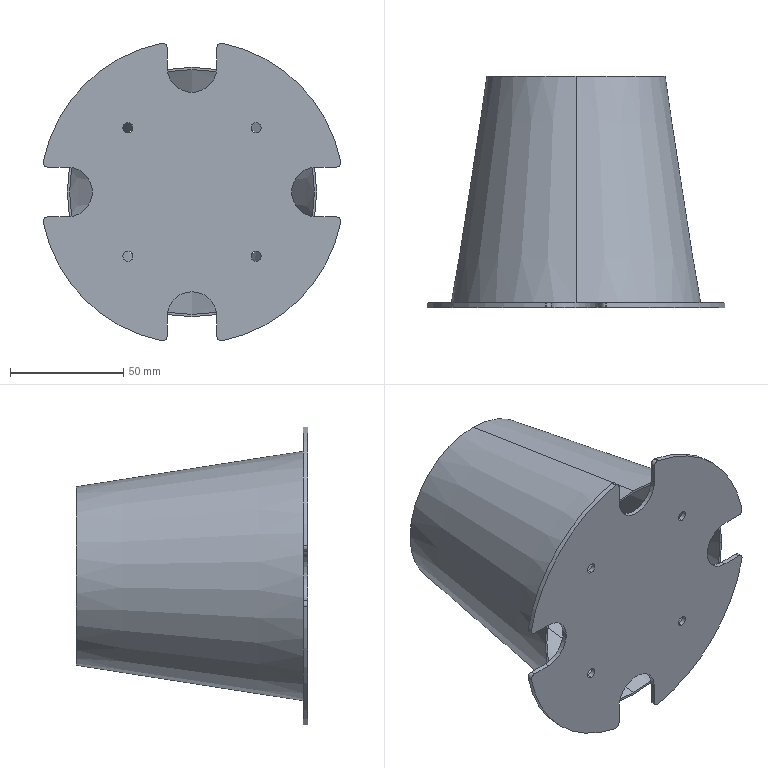Part | SolidWorks | features BaseBody 2 | 2 solids | 43 faces | box 131.373 x 102 x 131.373 mm | volume 54164 mm3 | cylinder 27 | plane 12 | cone 4 | commonest cylinder face diameters 4 x10 4.5 x8 22 x5 134 x4
STEP:
#1=CARTESIAN_POINT('',(0.,100.,38.363));
#2=VERTEX_POINT('',#1);
#3=CARTESIAN_POINT('',(0.,0.,53.988));
#4=VERTEX_POINT('',#3);
#5=CARTESIAN_POINT('',(0.,99.846,38.387));
#6=DIRECTION('',(0.,-0.988,0.1544));
#7=VECTOR('',#6,1000.);
#8=LINE('',#5,#7);
#9=EDGE_CURVE('',#2,#4,#8,.T.);
#10=ORIENTED_EDGE('',*,*,#9,.F.);
#11=CARTESIAN_POINT('',(0.,100.,-38.363));
#12=VERTEX_POINT('',#11);
#13=CARTESIAN_POINT('',(0.,100.,0.));
#14=DIRECTION('',(0.,1.,0.));
#15=DIRECTION('',(0.,0.,1.));
#16=AXIS2_PLACEMENT_3D('',#13,#14,#15);
#17=CIRCLE('',#16,38.363);
#18=EDGE_CURVE('',#2,#12,#17,.T.);
#19=ORIENTED_EDGE('',*,*,#18,.T.);
#20=CARTESIAN_POINT('',(0.,0.,-53.988));
#21=VERTEX_POINT('',#20);
#22=CARTESIAN_POINT('',(0.,99.846,-38.387));
#23=DIRECTION('',(0.,-0.988,-0.1544));
#24=VECTOR('',#23,1000.);
#25=LINE('',#22,#24);
#26=EDGE_CURVE('',#12,#21,#25,.T.);
#27=ORIENTED_EDGE('',*,*,#26,.T.);
#28=CARTESIAN_POINT('',(0.,0.,0.));
#29=DIRECTION('',(0.,1.,0.));
#30=DIRECTION('',(0.,0.,-1.));
#31=AXIS2_PLACEMENT_3D('',#28,#29,#30);
#32=CIRCLE('',#31,53.988);
#33=EDGE_CURVE('',#4,#21,#32,.T.);
#34=ORIENTED_EDGE('',*,*,#33,.F.);
#35=EDGE_LOOP('',(#10,#19,#27,#34));
#36=FACE_OUTER_BOUND('',#35,.T.);
#37=CARTESIAN_POINT('',(0.,99.846,0.));
#38=DIRECTION('',(0.,-1.,0.));
#39=DIRECTION('',(0.,0.,-1.));
#40=AXIS2_PLACEMENT_3D('',#37,#38,#39);
#41=CONICAL_SURFACE('',#40,38.387,0.155);
#42=ADVANCED_FACE('',(#36),#41,.F.);
#43=CARTESIAN_POINT('',(0.,100.,39.375));
#44=VERTEX_POINT('',#43);
#45=CARTESIAN_POINT('',(0.,0.,55.));
#46=VERTEX_POINT('',#45);
#47=CARTESIAN_POINT('',(0.,100.,39.375));
#48=DIRECTION('',(0.,-0.988,0.1544));
#49=VECTOR('',#48,1000.);
#50=LINE('',#47,#49);
#51=EDGE_CURVE('',#44,#46,#50,.T.);
#52=ORIENTED_EDGE('',*,*,#51,.F.);
#53=CARTESIAN_POINT('',(0.,100.,-39.375));
#54=VERTEX_POINT('',#53);
#55=CARTESIAN_POINT('',(0.,100.,0.));
#56=DIRECTION('',(0.,1.,0.));
#57=DIRECTION('',(0.,0.,1.));
#58=AXIS2_PLACEMENT_3D('',#55,#56,#57);
#59=CIRCLE('',#58,39.375);
#60=EDGE_CURVE('',#54,#44,#59,.T.);
#61=ORIENTED_EDGE('',*,*,#60,.F.);
#62=CARTESIAN_POINT('',(0.,0.,-55.));
#63=VERTEX_POINT('',#62);
#64=CARTESIAN_POINT('',(0.,100.,-39.375));
#65=DIRECTION('',(0.,-0.988,-0.1544));
#66=VECTOR('',#65,1000.);
#67=LINE('',#64,#66);
#68=EDGE_CURVE('',#54,#63,#67,.T.);
#69=ORIENTED_EDGE('',*,*,#68,.T.);
#70=CARTESIAN_POINT('',(0.,0.,0.));
#71=DIRECTION('',(0.,1.,0.));
#72=DIRECTION('',(0.,0.,1.));
#73=AXIS2_PLACEMENT_3D('',#70,#71,#72);
#74=CIRCLE('',#73,55.);
#75=EDGE_CURVE('',#63,#46,#74,.T.);
#76=ORIENTED_EDGE('',*,*,#75,.T.);
#77=EDGE_LOOP('',(#52,#61,#69,#76));
#78=FACE_OUTER_BOUND('',#77,.T.);
#79=CARTESIAN_POINT('',(0.,100.,0.));
#80=DIRECTION('',(0.,-1.,0.));
#81=DIRECTION('',(0.,0.,-1.));
#82=AXIS2_PLACEMENT_3D('',#79,#80,#81);
#83=CONICAL_SURFACE('',#82,39.375,0.155);
#84=ADVANCED_FACE('',(#78),#83,.T.);
#85=CARTESIAN_POINT('',(0.,100.,0.));
#86=DIRECTION('',(0.,1.,0.));
#87=DIRECTION('',(0.,0.,1.));
#88=AXIS2_PLACEMENT_3D('',#85,#86,#87);
#89=CIRCLE('',#88,38.363);
#90=EDGE_CURVE('',#12,#2,#89,.T.);
#91=ORIENTED_EDGE('',*,*,#90,.F.);
#92=ORIENTED_EDGE('',*,*,#18,.F.);
#93=EDGE_LOOP('',(#91,#92));
#94=FACE_BOUND('',#93,.T.);
#95=ORIENTED_EDGE('',*,*,#60,.T.);
#96=CARTESIAN_POINT('',(0.,100.,0.));
#97=DIRECTION('',(0.,1.,0.));
#98=DIRECTION('',(0.,0.,1.));
#99=AXIS2_PLACEMENT_3D('',#96,#97,#98);
#100=CIRCLE('',#99,39.375);
#101=EDGE_CURVE('',#44,#54,#100,.T.);
#102=ORIENTED_EDGE('',*,*,#101,.T.);
#103=EDGE_LOOP('',(#95,#102));
#104=FACE_OUTER_BOUND('',#103,.T.);
#105=CARTESIAN_POINT('',(-39.375,100.,0.));
#106=DIRECTION('',(0.,1.,0.));
#107=DIRECTION('',(1.,0.,0.));
#108=AXIS2_PLACEMENT_3D('',#105,#106,#107);
#109=PLANE('',#108);
#110=ADVANCED_FACE('',(#94,#104),#109,.T.);
#111=CARTESIAN_POINT('',(0.,0.,0.));
#112=DIRECTION('',(0.,1.,0.));
#113=DIRECTION('',(0.,0.,-1.));
#114=AXIS2_PLACEMENT_3D('',#111,#112,#113);
#115=CIRCLE('',#114,53.988);
#116=EDGE_CURVE('',#21,#4,#115,.T.);
#117=ORIENTED_EDGE('',*,*,#116,.T.);
#118=ORIENTED_EDGE('',*,*,#33,.T.);
#119=EDGE_LOOP('',(#117,#118));
#120=FACE_BOUND('',#119,.T.);
#121=ORIENTED_EDGE('',*,*,#75,.F.);
#122=CARTESIAN_POINT('',(0.,0.,0.));
#123=DIRECTION('',(0.,1.,0.));
#124=DIRECTION('',(0.,0.,1.));
#125=AXIS2_PLACEMENT_3D('',#122,#123,#124);
#126=CIRCLE('',#125,55.);
#127=EDGE_CURVE('',#46,#63,#126,.T.);
#128=ORIENTED_EDGE('',*,*,#127,.F.);
#129=EDGE_LOOP('',(#121,#128));
#130=FACE_OUTER_BOUND('',#129,.T.);
#131=CARTESIAN_POINT('',(0.,0.,0.));
#132=DIRECTION('',(0.,-1.,0.));
#133=DIRECTION('',(0.,0.,-1.));
#134=AXIS2_PLACEMENT_3D('',#131,#132,#133);
#135=PLANE('',#134);
#136=ADVANCED_FACE('',(#120,#130),#135,.T.);
#137=ORIENTED_EDGE('',*,*,#101,.F.);
#138=ORIENTED_EDGE('',*,*,#51,.T.);
#139=ORIENTED_EDGE('',*,*,#127,.T.);
#140=ORIENTED_EDGE('',*,*,#68,.F.);
#141=EDGE_LOOP('',(#137,#138,#139,#140));
#142=FACE_OUTER_BOUND('',#141,.T.);
#143=CARTESIAN_POINT('',(0.,100.,0.));
#144=DIRECTION('',(0.,-1.,0.));
#145=DIRECTION('',(0.,0.,-1.));
#146=AXIS2_PLACEMENT_3D('',#143,#144,#145);
#147=CONICAL_SURFACE('',#146,39.375,0.155);
#148=ADVANCED_FACE('',(#142),#147,.T.);
#149=ORIENTED_EDGE('',*,*,#90,.T.);
#150=ORIENTED_EDGE('',*,*,#9,.T.);
#151=ORIENTED_EDGE('',*,*,#116,.F.);
#152=ORIENTED_EDGE('',*,*,#26,.F.);
#153=EDGE_LOOP('',(#149,#150,#151,#152));
#154=FACE_OUTER_BOUND('',#153,.T.);
#155=CARTESIAN_POINT('',(0.,99.846,0.));
#156=DIRECTION('',(0.,-1.,0.));
#157=DIRECTION('',(0.,0.,-1.));
#158=AXIS2_PLACEMENT_3D('',#155,#156,#157);
#159=CONICAL_SURFACE('',#158,38.387,0.155);
#160=ADVANCED_FACE('',(#154),#159,.F.);
#161=CLOSED_SHELL('',(#42,#84,#110,#136,#148,#160));
#162=MANIFOLD_SOLID_BREP('',#161);
#163=CARTESIAN_POINT('',(13.4,0.,-65.646));
#164=VERTEX_POINT('',#163);
#165=CARTESIAN_POINT('',(11.,0.,-63.687));
#166=VERTEX_POINT('',#165);
#167=CARTESIAN_POINT('',(13.,0.,-63.687));
#168=DIRECTION('',(0.,1.,0.));
#169=DIRECTION('',(0.,0.,-1.));
#170=AXIS2_PLACEMENT_3D('',#167,#168,#169);
#171=CIRCLE('',#170,2.);
#172=EDGE_CURVE('',#164,#166,#171,.T.);
#173=ORIENTED_EDGE('',*,*,#172,.F.);
#174=CARTESIAN_POINT('',(13.4,-2.,-65.646));
#175=VERTEX_POINT('',#174);
#176=CARTESIAN_POINT('',(13.4,-2.,-65.646));
#177=DIRECTION('',(0.,1.,0.));
#178=VECTOR('',#177,1000.);
#179=LINE('',#176,#178);
#180=EDGE_CURVE('',#175,#164,#179,.T.);
#181=ORIENTED_EDGE('',*,*,#180,.F.);
#182=CARTESIAN_POINT('',(11.,-2.,-63.687));
#183=VERTEX_POINT('',#182);
#184=CARTESIAN_POINT('',(13.,-2.,-63.687));
#185=DIRECTION('',(0.,-1.,0.));
#186=DIRECTION('',(0.,0.,-1.));
#187=AXIS2_PLACEMENT_3D('',#184,#185,#186);
#188=CIRCLE('',#187,2.);
#189=EDGE_CURVE('',#183,#175,#188,.T.);
#190=ORIENTED_EDGE('',*,*,#189,.F.);
#191=CARTESIAN_POINT('',(11.,-2.001,-63.687));
#192=DIRECTION('',(0.,-1.,0.));
#193=VECTOR('',#192,1000.);
#194=LINE('',#191,#193);
#195=EDGE_CURVE('',#166,#183,#194,.T.);
#196=ORIENTED_EDGE('',*,*,#195,.F.);
#197=EDGE_LOOP('',(#173,#181,#190,#196));
#198=FACE_OUTER_BOUND('',#197,.T.);
#199=CARTESIAN_POINT('',(13.,-2.,-63.687));
#200=DIRECTION('',(0.,1.,0.));
#201=DIRECTION('',(0.,0.,1.));
#202=AXIS2_PLACEMENT_3D('',#199,#200,#201);
#203=CYLINDRICAL_SURFACE('',#202,2.);
#204=ADVANCED_FACE('',(#198),#203,.T.);
#205=CARTESIAN_POINT('',(-13.4,-2.,-65.646));
#206=VERTEX_POINT('',#205);
#207=CARTESIAN_POINT('',(-11.,-2.,-63.687));
#208=VERTEX_POINT('',#207);
#209=CARTESIAN_POINT('',(-13.,-2.,-63.687));
#210=DIRECTION('',(0.,-1.,0.));
#211=DIRECTION('',(0.,0.,-1.));
#212=AXIS2_PLACEMENT_3D('',#209,#210,#211);
#213=CIRCLE('',#212,2.);
#214=EDGE_CURVE('',#206,#208,#213,.T.);
#215=ORIENTED_EDGE('',*,*,#214,.F.);
#216=CARTESIAN_POINT('',(-13.4,0.,-65.646));
#217=VERTEX_POINT('',#216);
#218=CARTESIAN_POINT('',(-13.4,-2.,-65.646));
#219=DIRECTION('',(0.,-1.,0.));
#220=VECTOR('',#219,1000.);
#221=LINE('',#218,#220);
#222=EDGE_CURVE('',#217,#206,#221,.T.);
#223=ORIENTED_EDGE('',*,*,#222,.F.);
#224=CARTESIAN_POINT('',(-11.,0.,-63.687));
#225=VERTEX_POINT('',#224);
#226=CARTESIAN_POINT('',(-13.,0.,-63.687));
#227=DIRECTION('',(0.,1.,0.));
#228=DIRECTION('',(0.,0.,-1.));
#229=AXIS2_PLACEMENT_3D('',#226,#227,#228);
#230=CIRCLE('',#229,2.);
#231=EDGE_CURVE('',#225,#217,#230,.T.);
#232=ORIENTED_EDGE('',*,*,#231,.F.);
#233=CARTESIAN_POINT('',(-11.,-2.001,-63.687));
#234=DIRECTION('',(0.,1.,0.));
#235=VECTOR('',#234,1000.);
#236=LINE('',#233,#235);
#237=EDGE_CURVE('',#208,#225,#236,.T.);
#238=ORIENTED_EDGE('',*,*,#237,.F.);
#239=EDGE_LOOP('',(#215,#223,#232,#238));
#240=FACE_OUTER_BOUND('',#239,.T.);
#241=CARTESIAN_POINT('',(-13.,-2.,-63.687));
#242=DIRECTION('',(0.,1.,0.));
#243=DIRECTION('',(0.,0.,1.));
#244=AXIS2_PLACEMENT_3D('',#241,#242,#243);
#245=CYLINDRICAL_SURFACE('',#244,2.);
#246=ADVANCED_FACE('',(#240),#245,.T.);
#247=CARTESIAN_POINT('',(65.646,-2.,-13.4));
#248=VERTEX_POINT('',#247);
#249=CARTESIAN_POINT('',(63.687,-2.,-11.));
#250=VERTEX_POINT('',#249);
#251=CARTESIAN_POINT('',(63.687,-2.,-13.));
#252=DIRECTION('',(0.,-1.,0.));
#253=DIRECTION('',(0.,0.,-1.));
#254=AXIS2_PLACEMENT_3D('',#251,#252,#253);
#255=CIRCLE('',#254,2.);
#256=EDGE_CURVE('',#248,#250,#255,.T.);
#257=ORIENTED_EDGE('',*,*,#256,.F.);
#258=CARTESIAN_POINT('',(65.646,0.,-13.4));
#259=VERTEX_POINT('',#258);
#260=CARTESIAN_POINT('',(65.646,-2.,-13.4));
#261=DIRECTION('',(0.,-1.,0.));
#262=VECTOR('',#261,1000.);
#263=LINE('',#260,#262);
#264=EDGE_CURVE('',#259,#248,#263,.T.);
#265=ORIENTED_EDGE('',*,*,#264,.F.);
#266=CARTESIAN_POINT('',(63.687,0.,-11.));
#267=VERTEX_POINT('',#266);
#268=CARTESIAN_POINT('',(63.687,0.,-13.));
#269=DIRECTION('',(0.,1.,0.));
#270=DIRECTION('',(0.,0.,-1.));
#271=AXIS2_PLACEMENT_3D('',#268,#269,#270);
#272=CIRCLE('',#271,2.);
#273=EDGE_CURVE('',#267,#259,#272,.T.);
#274=ORIENTED_EDGE('',*,*,#273,.F.);
#275=CARTESIAN_POINT('',(63.687,-2.001,-11.));
#276=DIRECTION('',(0.,1.,0.));
#277=VECTOR('',#276,1000.);
#278=LINE('',#275,#277);
#279=EDGE_CURVE('',#250,#267,#278,.T.);
#280=ORIENTED_EDGE('',*,*,#279,.F.);
#281=EDGE_LOOP('',(#257,#265,#274,#280));
#282=FACE_OUTER_BOUND('',#281,.T.);
#283=CARTESIAN_POINT('',(63.687,-2.,-13.));
#284=DIRECTION('',(0.,1.,0.));
#285=DIRECTION('',(0.,0.,1.));
#286=AXIS2_PLACEMENT_3D('',#283,#284,#285);
#287=CYLINDRICAL_SURFACE('',#286,2.);
#288=ADVANCED_FACE('',(#282),#287,.T.);
#289=CARTESIAN_POINT('',(65.646,0.,13.4));
#290=VERTEX_POINT('',#289);
#291=CARTESIAN_POINT('',(63.687,0.,11.));
#292=VERTEX_POINT('',#291);
#293=CARTESIAN_POINT('',(63.687,0.,13.));
#294=DIRECTION('',(0.,1.,0.));
#295=DIRECTION('',(0.,0.,-1.));
#296=AXIS2_PLACEMENT_3D('',#293,#294,#295);
#297=CIRCLE('',#296,2.);
#298=EDGE_CURVE('',#290,#292,#297,.T.);
#299=ORIENTED_EDGE('',*,*,#298,.F.);
#300=CARTESIAN_POINT('',(65.646,-2.,13.4));
#301=VERTEX_POINT('',#300);
#302=CARTESIAN_POINT('',(65.646,-2.,13.4));
#303=DIRECTION('',(0.,1.,0.));
#304=VECTOR('',#303,1000.);
#305=LINE('',#302,#304);
#306=EDGE_CURVE('',#301,#290,#305,.T.);
#307=ORIENTED_EDGE('',*,*,#306,.F.);
#308=CARTESIAN_POINT('',(63.687,-2.,11.));
#309=VERTEX_POINT('',#308);
#310=CARTESIAN_POINT('',(63.687,-2.,13.));
#311=DIRECTION('',(0.,-1.,0.));
#312=DIRECTION('',(0.,0.,-1.));
#313=AXIS2_PLACEMENT_3D('',#310,#311,#312);
#314=CIRCLE('',#313,2.);
#315=EDGE_CURVE('',#309,#301,#314,.T.);
#316=ORIENTED_EDGE('',*,*,#315,.F.);
#317=CARTESIAN_POINT('',(63.687,-2.001,11.));
#318=DIRECTION('',(0.,-1.,0.));
#319=VECTOR('',#318,1000.);
#320=LINE('',#317,#319);
#321=EDGE_CURVE('',#292,#309,#320,.T.);
#322=ORIENTED_EDGE('',*,*,#321,.F.);
#323=EDGE_LOOP('',(#299,#307,#316,#322));
#324=FACE_OUTER_BOUND('',#323,.T.);
#325=CARTESIAN_POINT('',(63.687,-2.,13.));
#326=DIRECTION('',(0.,1.,0.));
#327=DIRECTION('',(0.,0.,1.));
#328=AXIS2_PLACEMENT_3D('',#325,#326,#327);
#329=CYLINDRICAL_SURFACE('',#328,2.);
#330=ADVANCED_FACE('',(#324),#329,.T.);
#331=CARTESIAN_POINT('',(-65.646,0.,-13.4));
#332=VERTEX_POINT('',#331);
#333=CARTESIAN_POINT('',(-63.687,0.,-11.));
#334=VERTEX_POINT('',#333);
#335=CARTESIAN_POINT('',(-63.687,0.,-13.));
#336=DIRECTION('',(0.,1.,0.));
#337=DIRECTION('',(0.,0.,-1.));
#338=AXIS2_PLACEMENT_3D('',#335,#336,#337);
#339=CIRCLE('',#338,2.);
#340=EDGE_CURVE('',#332,#334,#339,.T.);
#341=ORIENTED_EDGE('',*,*,#340,.F.);
#342=CARTESIAN_POINT('',(-65.646,-2.,-13.4));
#343=VERTEX_POINT('',#342);
#344=CARTESIAN_POINT('',(-65.646,-2.,-13.4));
#345=DIRECTION('',(0.,1.,0.));
#346=VECTOR('',#345,1000.);
#347=LINE('',#344,#346);
#348=EDGE_CURVE('',#343,#332,#347,.T.);
#349=ORIENTED_EDGE('',*,*,#348,.F.);
#350=CARTESIAN_POINT('',(-63.687,-2.,-11.));
#351=VERTEX_POINT('',#350);
#352=CARTESIAN_POINT('',(-63.687,-2.,-13.));
#353=DIRECTION('',(0.,-1.,0.));
#354=DIRECTION('',(0.,0.,-1.));
#355=AXIS2_PLACEMENT_3D('',#352,#353,#354);
#356=CIRCLE('',#355,2.);
#357=EDGE_CURVE('',#351,#343,#356,.T.);
#358=ORIENTED_EDGE('',*,*,#357,.F.);
#359=CARTESIAN_POINT('',(-63.687,-2.001,-11.));
#360=DIRECTION('',(0.,-1.,0.));
#361=VECTOR('',#360,1000.);
#362=LINE('',#359,#361);
#363=EDGE_CURVE('',#334,#351,#362,.T.);
#364=ORIENTED_EDGE('',*,*,#363,.F.);
#365=EDGE_LOOP('',(#341,#349,#358,#364));
#366=FACE_OUTER_BOUND('',#365,.T.);
#367=CARTESIAN_POINT('',(-63.687,-2.,-13.));
#368=DIRECTION('',(0.,1.,0.));
#369=DIRECTION('',(0.,0.,1.));
#370=AXIS2_PLACEMENT_3D('',#367,#368,#369);
#371=CYLINDRICAL_SURFACE('',#370,2.);
#372=ADVANCED_FACE('',(#366),#371,.T.);
#373=CARTESIAN_POINT('',(-65.646,-2.,13.4));
#374=VERTEX_POINT('',#373);
#375=CARTESIAN_POINT('',(-63.687,-2.,11.));
#376=VERTEX_POINT('',#375);
#377=CARTESIAN_POINT('',(-63.687,-2.,13.));
#378=DIRECTION('',(0.,-1.,0.));
#379=DIRECTION('',(0.,0.,-1.));
#380=AXIS2_PLACEMENT_3D('',#377,#378,#379);
#381=CIRCLE('',#380,2.);
#382=EDGE_CURVE('',#374,#376,#381,.T.);
#383=ORIENTED_EDGE('',*,*,#382,.F.);
#384=CARTESIAN_POINT('',(-65.646,0.,13.4));
#385=VERTEX_POINT('',#384);
#386=CARTESIAN_POINT('',(-65.646,-2.,13.4));
#387=DIRECTION('',(0.,-1.,0.));
#388=VECTOR('',#387,1000.);
#389=LINE('',#386,#388);
#390=EDGE_CURVE('',#385,#374,#389,.T.);
#391=ORIENTED_EDGE('',*,*,#390,.F.);
#392=CARTESIAN_POINT('',(-63.687,0.,11.));
#393=VERTEX_POINT('',#392);
#394=CARTESIAN_POINT('',(-63.687,0.,13.));
#395=DIRECTION('',(0.,1.,0.));
#396=DIRECTION('',(0.,0.,-1.));
#397=AXIS2_PLACEMENT_3D('',#394,#395,#396);
#398=CIRCLE('',#397,2.);
#399=EDGE_CURVE('',#393,#385,#398,.T.);
#400=ORIENTED_EDGE('',*,*,#399,.F.);
#401=CARTESIAN_POINT('',(-63.687,-2.001,11.));
#402=DIRECTION('',(0.,1.,0.));
#403=VECTOR('',#402,1000.);
#404=LINE('',#401,#403);
#405=EDGE_CURVE('',#376,#393,#404,.T.);
#406=ORIENTED_EDGE('',*,*,#405,.F.);
#407=EDGE_LOOP('',(#383,#391,#400,#406));
#408=FACE_OUTER_BOUND('',#407,.T.);
#409=CARTESIAN_POINT('',(-63.687,-2.,13.));
#410=DIRECTION('',(0.,1.,0.));
#411=DIRECTION('',(0.,0.,1.));
#412=AXIS2_PLACEMENT_3D('',#409,#410,#411);
#413=CYLINDRICAL_SURFACE('',#412,2.);
#414=ADVANCED_FACE('',(#408),#413,.T.);
#415=CARTESIAN_POINT('',(13.,-2.,65.687));
#416=VERTEX_POINT('',#415);
#417=CARTESIAN_POINT('',(13.,0.,65.687));
#418=VERTEX_POINT('',#417);
#419=CARTESIAN_POINT('',(13.,-2.,65.687));
#420=DIRECTION('',(0.,1.,0.));
#421=VECTOR('',#420,1000.);
#422=LINE('',#419,#421);
#423=EDGE_CURVE('',#416,#418,#422,.T.);
#424=ORIENTED_EDGE('',*,*,#423,.F.);
#425=CARTESIAN_POINT('',(13.4,-2.,65.646));
#426=VERTEX_POINT('',#425);
#427=CARTESIAN_POINT('',(13.,-2.,63.687));
#428=DIRECTION('',(0.,-1.,0.));
#429=DIRECTION('',(0.,0.,-1.));
#430=AXIS2_PLACEMENT_3D('',#427,#428,#429);
#431=CIRCLE('',#430,2.);
#432=EDGE_CURVE('',#426,#416,#431,.T.);
#433=ORIENTED_EDGE('',*,*,#432,.F.);
#434=CARTESIAN_POINT('',(13.4,0.,65.646));
#435=VERTEX_POINT('',#434);
#436=CARTESIAN_POINT('',(13.4,-2.,65.646));
#437=DIRECTION('',(0.,-1.,0.));
#438=VECTOR('',#437,1000.);
#439=LINE('',#436,#438);
#440=EDGE_CURVE('',#435,#426,#439,.T.);
#441=ORIENTED_EDGE('',*,*,#440,.F.);
#442=CARTESIAN_POINT('',(13.,0.,63.687));
#443=DIRECTION('',(0.,1.,0.));
#444=DIRECTION('',(0.,0.,-1.));
#445=AXIS2_PLACEMENT_3D('',#442,#443,#444);
#446=CIRCLE('',#445,2.);
#447=EDGE_CURVE('',#418,#435,#446,.T.);
#448=ORIENTED_EDGE('',*,*,#447,.F.);
#449=EDGE_LOOP('',(#424,#433,#441,#448));
#450=FACE_OUTER_BOUND('',#449,.T.);
#451=CARTESIAN_POINT('',(13.,-2.,63.687));
#452=DIRECTION('',(0.,1.,0.));
#453=DIRECTION('',(0.,0.,1.));
#454=AXIS2_PLACEMENT_3D('',#451,#452,#453);
#455=CYLINDRICAL_SURFACE('',#454,2.);
#456=ADVANCED_FACE('',(#450),#455,.T.);
#457=CARTESIAN_POINT('',(-13.,-2.,65.687));
#458=VERTEX_POINT('',#457);
#459=CARTESIAN_POINT('',(-13.,0.,65.687));
#460=VERTEX_POINT('',#459);
#461=CARTESIAN_POINT('',(-13.,-2.,65.687));
#462=DIRECTION('',(0.,1.,0.));
#463=VECTOR('',#462,1000.);
#464=LINE('',#461,#463);
#465=EDGE_CURVE('',#458,#460,#464,.T.);
#466=ORIENTED_EDGE('',*,*,#465,.F.);
#467=CARTESIAN_POINT('',(-11.,-2.,63.687));
#468=VERTEX_POINT('',#467);
#469=CARTESIAN_POINT('',(-13.,-2.,63.687));
#470=DIRECTION('',(0.,-1.,0.));
#471=DIRECTION('',(0.,0.,-1.));
#472=AXIS2_PLACEMENT_3D('',#469,#470,#471);
#473=CIRCLE('',#472,2.);
#474=EDGE_CURVE('',#468,#458,#473,.T.);
#475=ORIENTED_EDGE('',*,*,#474,.F.);
#476=CARTESIAN_POINT('',(-11.,0.,63.687));
#477=VERTEX_POINT('',#476);
#478=CARTESIAN_POINT('',(-11.,-2.001,63.687));
#479=DIRECTION('',(0.,-1.,0.));
#480=VECTOR('',#479,1000.);
#481=LINE('',#478,#480);
#482=EDGE_CURVE('',#477,#468,#481,.T.);
#483=ORIENTED_EDGE('',*,*,#482,.F.);
#484=CARTESIAN_POINT('',(-13.,0.,63.687));
#485=DIRECTION('',(0.,1.,0.));
#486=DIRECTION('',(0.,0.,-1.));
#487=AXIS2_PLACEMENT_3D('',#484,#485,#486);
#488=CIRCLE('',#487,2.);
#489=EDGE_CURVE('',#460,#477,#488,.T.);
#490=ORIENTED_EDGE('',*,*,#489,.F.);
#491=EDGE_LOOP('',(#466,#475,#483,#490));
#492=FACE_OUTER_BOUND('',#491,.T.);
#493=CARTESIAN_POINT('',(-13.,-2.,63.687));
#494=DIRECTION('',(0.,1.,0.));
#495=DIRECTION('',(0.,0.,1.));
#496=AXIS2_PLACEMENT_3D('',#493,#494,#495);
#497=CYLINDRICAL_SURFACE('',#496,2.);
#498=ADVANCED_FACE('',(#492),#497,.T.);
#499=CARTESIAN_POINT('',(55.,-2.,-11.));
#500=VERTEX_POINT('',#499);
#501=CARTESIAN_POINT('',(55.,0.,-11.));
#502=VERTEX_POINT('',#501);
#503=CARTESIAN_POINT('',(55.,-2.001,-11.));
#504=DIRECTION('',(0.,1.,0.));
#505=VECTOR('',#504,1000.);
#506=LINE('',#503,#505);
#507=EDGE_CURVE('',#500,#502,#506,.T.);
#508=ORIENTED_EDGE('',*,*,#507,.T.);
#509=CARTESIAN_POINT('',(55.,0.,11.));
#510=VERTEX_POINT('',#509);
#511=CARTESIAN_POINT('',(55.,0.,0.));
#512=DIRECTION('',(0.,1.,0.));
#513=DIRECTION('',(-1.,0.,0.));
#514=AXIS2_PLACEMENT_3D('',#511,#512,#513);
#515=CIRCLE('',#514,11.);
#516=EDGE_CURVE('',#502,#510,#515,.T.);
#517=ORIENTED_EDGE('',*,*,#516,.T.);
#518=CARTESIAN_POINT('',(55.,-2.,11.));
#519=VERTEX_POINT('',#518);
#520=CARTESIAN_POINT('',(55.,-2.001,11.));
#521=DIRECTION('',(0.,1.,0.));
#522=VECTOR('',#521,1000.);
#523=LINE('',#520,#522);
#524=EDGE_CURVE('',#519,#510,#523,.T.);
#525=ORIENTED_EDGE('',*,*,#524,.F.);
#526=CARTESIAN_POINT('',(55.,-2.,0.));
#527=DIRECTION('',(0.,1.,0.));
#528=DIRECTION('',(0.,0.,-1.));
#529=AXIS2_PLACEMENT_3D('',#526,#527,#528);
#530=CIRCLE('',#529,11.);
#531=EDGE_CURVE('',#500,#519,#530,.T.);
#532=ORIENTED_EDGE('',*,*,#531,.F.);
#533=EDGE_LOOP('',(#508,#517,#525,#532));
#534=FACE_OUTER_BOUND('',#533,.T.);
#535=CARTESIAN_POINT('',(55.,-2.001,0.));
#536=DIRECTION('',(0.,1.,0.));
#537=DIRECTION('',(0.,0.,1.));
#538=AXIS2_PLACEMENT_3D('',#535,#536,#537);
#539=CYLINDRICAL_SURFACE('',#538,11.);
#540=ADVANCED_FACE('',(#534),#539,.F.);
#541=CARTESIAN_POINT('',(67.,-2.,-11.));
#542=DIRECTION('',(-1.,0.,0.));
#543=VECTOR('',#542,1000.);
#544=LINE('',#541,#543);
#545=EDGE_CURVE('',#250,#500,#544,.T.);
#546=ORIENTED_EDGE('',*,*,#545,.F.);
#547=ORIENTED_EDGE('',*,*,#279,.T.);
#548=CARTESIAN_POINT('',(67.,0.,-11.));
#549=DIRECTION('',(-1.,0.,0.));
#550=VECTOR('',#549,1000.);
#551=LINE('',#548,#550);
#552=EDGE_CURVE('',#267,#502,#551,.T.);
#553=ORIENTED_EDGE('',*,*,#552,.T.);
#554=ORIENTED_EDGE('',*,*,#507,.F.);
#555=EDGE_LOOP('',(#546,#547,#553,#554));
#556=FACE_OUTER_BOUND('',#555,.T.);
#557=CARTESIAN_POINT('',(67.,-2.001,-11.));
#558=DIRECTION('',(0.,0.,-1.));
#559=DIRECTION('',(0.,-1.,0.));
#560=AXIS2_PLACEMENT_3D('',#557,#558,#559);
#561=PLANE('',#560);
#562=ADVANCED_FACE('',(#556),#561,.F.);
#563=CARTESIAN_POINT('',(67.,0.,11.));
#564=DIRECTION('',(1.,0.,0.));
#565=VECTOR('',#564,1000.);
#566=LINE('',#563,#565);
#567=EDGE_CURVE('',#510,#292,#566,.T.);
#568=ORIENTED_EDGE('',*,*,#567,.T.);
#569=ORIENTED_EDGE('',*,*,#321,.T.);
#570=CARTESIAN_POINT('',(67.,-2.,11.));
#571=DIRECTION('',(1.,0.,0.));
#572=VECTOR('',#571,1000.);
#573=LINE('',#570,#572);
#574=EDGE_CURVE('',#519,#309,#573,.T.);
#575=ORIENTED_EDGE('',*,*,#574,.F.);
#576=ORIENTED_EDGE('',*,*,#524,.T.);
#577=EDGE_LOOP('',(#568,#569,#575,#576));
#578=FACE_OUTER_BOUND('',#577,.T.);
#579=CARTESIAN_POINT('',(67.,-2.001,11.));
#580=DIRECTION('',(0.,0.,1.));
#581=DIRECTION('',(1.,0.,0.));
#582=AXIS2_PLACEMENT_3D('',#579,#580,#581);
#583=PLANE('',#582);
#584=ADVANCED_FACE('',(#578),#583,.F.);
#585=CARTESIAN_POINT('',(11.,-2.,55.));
#586=VERTEX_POINT('',#585);
#587=CARTESIAN_POINT('',(11.,0.,55.));
#588=VERTEX_POINT('',#587);
#589=CARTESIAN_POINT('',(11.,-2.001,55.));
#590=DIRECTION('',(0.,1.,0.));
#591=VECTOR('',#590,1000.);
#592=LINE('',#589,#591);
#593=EDGE_CURVE('',#586,#588,#592,.T.);
#594=ORIENTED_EDGE('',*,*,#593,.T.);
#595=CARTESIAN_POINT('',(-11.,0.,55.));
#596=VERTEX_POINT('',#595);
#597=CARTESIAN_POINT('',(0.,0.,55.));
#598=DIRECTION('',(0.,1.,0.));
#599=DIRECTION('',(0.,0.,-1.));
#600=AXIS2_PLACEMENT_3D('',#597,#598,#599);
#601=CIRCLE('',#600,11.);
#602=EDGE_CURVE('',#588,#596,#601,.T.);
#603=ORIENTED_EDGE('',*,*,#602,.T.);
#604=CARTESIAN_POINT('',(-11.,-2.,55.));
#605=VERTEX_POINT('',#604);
#606=CARTESIAN_POINT('',(-11.,-2.001,55.));
#607=DIRECTION('',(0.,1.,0.));
#608=VECTOR('',#607,1000.);
#609=LINE('',#606,#608);
#610=EDGE_CURVE('',#605,#596,#609,.T.);
#611=ORIENTED_EDGE('',*,*,#610,.F.);
#612=CARTESIAN_POINT('',(0.,-2.,55.));
#613=DIRECTION('',(0.,1.,0.));
#614=DIRECTION('',(0.,0.,-1.));
#615=AXIS2_PLACEMENT_3D('',#612,#613,#614);
#616=CIRCLE('',#615,11.);
#617=EDGE_CURVE('',#586,#605,#616,.T.);
#618=ORIENTED_EDGE('',*,*,#617,.F.);
#619=EDGE_LOOP('',(#594,#603,#611,#618));
#620=FACE_OUTER_BOUND('',#619,.T.);
#621=CARTESIAN_POINT('',(0.,-2.001,55.));
#622=DIRECTION('',(0.,1.,0.));
#623=DIRECTION('',(0.,0.,1.));
#624=AXIS2_PLACEMENT_3D('',#621,#622,#623);
#625=CYLINDRICAL_SURFACE('',#624,11.);
#626=ADVANCED_FACE('',(#620),#625,.F.);
#627=CARTESIAN_POINT('',(11.,-2.,63.687));
#628=VERTEX_POINT('',#627);
#629=CARTESIAN_POINT('',(11.,-2.,67.));
#630=DIRECTION('',(0.,0.,-1.));
#631=VECTOR('',#630,1000.);
#632=LINE('',#629,#631);
#633=EDGE_CURVE('',#628,#586,#632,.T.);
#634=ORIENTED_EDGE('',*,*,#633,.F.);
#635=CARTESIAN_POINT('',(11.,0.,63.687));
#636=VERTEX_POINT('',#635);
#637=CARTESIAN_POINT('',(11.,-2.001,63.687));
#638=DIRECTION('',(0.,1.,0.));
#639=VECTOR('',#638,1000.);
#640=LINE('',#637,#639);
#641=EDGE_CURVE('',#628,#636,#640,.T.);
#642=ORIENTED_EDGE('',*,*,#641,.T.);
#643=CARTESIAN_POINT('',(11.,0.,67.));
#644=DIRECTION('',(0.,0.,-1.));
#645=VECTOR('',#644,1000.);
#646=LINE('',#643,#645);
#647=EDGE_CURVE('',#636,#588,#646,.T.);
#648=ORIENTED_EDGE('',*,*,#647,.T.);
#649=ORIENTED_EDGE('',*,*,#593,.F.);
#650=EDGE_LOOP('',(#634,#642,#648,#649));
#651=FACE_OUTER_BOUND('',#650,.T.);
#652=CARTESIAN_POINT('',(11.,-2.001,67.));
#653=DIRECTION('',(1.,0.,0.));
#654=DIRECTION('',(0.,1.,0.));
#655=AXIS2_PLACEMENT_3D('',#652,#653,#654);
#656=PLANE('',#655);
#657=ADVANCED_FACE('',(#651),#656,.F.);
#658=CARTESIAN_POINT('',(-11.,0.,67.));
#659=DIRECTION('',(0.,0.,1.));
#660=VECTOR('',#659,1000.);
#661=LINE('',#658,#660);
#662=EDGE_CURVE('',#596,#477,#661,.T.);
#663=ORIENTED_EDGE('',*,*,#662,.T.);
#664=ORIENTED_EDGE('',*,*,#482,.T.);
#665=CARTESIAN_POINT('',(-11.,-2.,67.));
#666=DIRECTION('',(0.,0.,1.));
#667=VECTOR('',#666,1000.);
#668=LINE('',#665,#667);
#669=EDGE_CURVE('',#605,#468,#668,.T.);
#670=ORIENTED_EDGE('',*,*,#669,.F.);
#671=ORIENTED_EDGE('',*,*,#610,.T.);
#672=EDGE_LOOP('',(#663,#664,#670,#671));
#673=FACE_OUTER_BOUND('',#672,.T.);
#674=CARTESIAN_POINT('',(-11.,-2.001,67.));
#675=DIRECTION('',(-1.,0.,0.));
#676=DIRECTION('',(0.,0.,1.));
#677=AXIS2_PLACEMENT_3D('',#674,#675,#676);
#678=PLANE('',#677);
#679=ADVANCED_FACE('',(#673),#678,.F.);
#680=CARTESIAN_POINT('',(-55.,-2.,11.));
#681=VERTEX_POINT('',#680);
#682=CARTESIAN_POINT('',(-55.,0.,11.));
#683=VERTEX_POINT('',#682);
#684=CARTESIAN_POINT('',(-55.,-2.001,11.));
#685=DIRECTION('',(0.,1.,0.));
#686=VECTOR('',#685,1000.);
#687=LINE('',#684,#686);
#688=EDGE_CURVE('',#681,#683,#687,.T.);
#689=ORIENTED_EDGE('',*,*,#688,.T.);
#690=CARTESIAN_POINT('',(-55.,0.,-11.));
#691=VERTEX_POINT('',#690);
#692=CARTESIAN_POINT('',(-55.,0.,0.));
#693=DIRECTION('',(0.,1.,0.));
#694=DIRECTION('',(1.,0.,0.));
#695=AXIS2_PLACEMENT_3D('',#692,#693,#694);
#696=CIRCLE('',#695,11.);
#697=EDGE_CURVE('',#683,#691,#696,.T.);
#698=ORIENTED_EDGE('',*,*,#697,.T.);
#699=CARTESIAN_POINT('',(-55.,-2.,-11.));
#700=VERTEX_POINT('',#699);
#701=CARTESIAN_POINT('',(-55.,-2.001,-11.));
#702=DIRECTION('',(0.,1.,0.));
#703=VECTOR('',#702,1000.);
#704=LINE('',#701,#703);
#705=EDGE_CURVE('',#700,#691,#704,.T.);
#706=ORIENTED_EDGE('',*,*,#705,.F.);
#707=CARTESIAN_POINT('',(-55.,-2.,0.));
#708=DIRECTION('',(0.,1.,0.));
#709=DIRECTION('',(0.,0.,-1.));
#710=AXIS2_PLACEMENT_3D('',#707,#708,#709);
#711=CIRCLE('',#710,11.);
#712=EDGE_CURVE('',#681,#700,#711,.T.);
#713=ORIENTED_EDGE('',*,*,#712,.F.);
#714=EDGE_LOOP('',(#689,#698,#706,#713));
#715=FACE_OUTER_BOUND('',#714,.T.);
#716=CARTESIAN_POINT('',(-55.,-2.001,0.));
#717=DIRECTION('',(0.,1.,0.));
#718=DIRECTION('',(0.,0.,1.));
#719=AXIS2_PLACEMENT_3D('',#716,#717,#718);
#720=CYLINDRICAL_SURFACE('',#719,11.);
#721=ADVANCED_FACE('',(#715),#720,.F.);
#722=CARTESIAN_POINT('',(-67.,-2.,11.));
#723=DIRECTION('',(1.,0.,0.));
#724=VECTOR('',#723,1000.);
#725=LINE('',#722,#724);
#726=EDGE_CURVE('',#376,#681,#725,.T.);
#727=ORIENTED_EDGE('',*,*,#726,.F.);
#728=ORIENTED_EDGE('',*,*,#405,.T.);
#729=CARTESIAN_POINT('',(-67.,0.,11.));
#730=DIRECTION('',(1.,0.,0.));
#731=VECTOR('',#730,1000.);
#732=LINE('',#729,#731);
#733=EDGE_CURVE('',#393,#683,#732,.T.);
#734=ORIENTED_EDGE('',*,*,#733,.T.);
#735=ORIENTED_EDGE('',*,*,#688,.F.);
#736=EDGE_LOOP('',(#727,#728,#734,#735));
#737=FACE_OUTER_BOUND('',#736,.T.);
#738=CARTESIAN_POINT('',(-67.,-2.001,11.));
#739=DIRECTION('',(0.,0.,1.));
#740=DIRECTION('',(1.,0.,0.));
#741=AXIS2_PLACEMENT_3D('',#738,#739,#740);
#742=PLANE('',#741);
#743=ADVANCED_FACE('',(#737),#742,.F.);
#744=CARTESIAN_POINT('',(-67.,0.,-11.));
#745=DIRECTION('',(-1.,0.,0.));
#746=VECTOR('',#745,1000.);
#747=LINE('',#744,#746);
#748=EDGE_CURVE('',#691,#334,#747,.T.);
#749=ORIENTED_EDGE('',*,*,#748,.T.);
#750=ORIENTED_EDGE('',*,*,#363,.T.);
#751=CARTESIAN_POINT('',(-67.,-2.,-11.));
#752=DIRECTION('',(-1.,0.,0.));
#753=VECTOR('',#752,1000.);
#754=LINE('',#751,#753);
#755=EDGE_CURVE('',#700,#351,#754,.T.);
#756=ORIENTED_EDGE('',*,*,#755,.F.);
#757=ORIENTED_EDGE('',*,*,#705,.T.);
#758=EDGE_LOOP('',(#749,#750,#756,#757));
#759=FACE_OUTER_BOUND('',#758,.T.);
#760=CARTESIAN_POINT('',(-67.,-2.001,-11.));
#761=DIRECTION('',(0.,0.,-1.));
#762=DIRECTION('',(0.,-1.,0.));
#763=AXIS2_PLACEMENT_3D('',#760,#761,#762);
#764=PLANE('',#763);
#765=ADVANCED_FACE('',(#759),#764,.F.);
#766=CARTESIAN_POINT('',(0.,-2.,-44.));
#767=VERTEX_POINT('',#766);
#768=CARTESIAN_POINT('',(0.,0.,-44.));
#769=VERTEX_POINT('',#768);
#770=CARTESIAN_POINT('',(0.,-2.001,-44.));
#771=DIRECTION('',(0.,1.,0.));
#772=VECTOR('',#771,1000.);
#773=LINE('',#770,#772);
#774=EDGE_CURVE('',#767,#769,#773,.T.);
#775=ORIENTED_EDGE('',*,*,#774,.F.);
#776=CARTESIAN_POINT('',(-11.,-2.,-55.));
#777=VERTEX_POINT('',#776);
#778=CARTESIAN_POINT('',(0.,-2.,-55.));
#779=DIRECTION('',(0.,1.,0.));
#780=DIRECTION('',(0.,0.,-1.));
#781=AXIS2_PLACEMENT_3D('',#778,#779,#780);
#782=CIRCLE('',#781,11.);
#783=EDGE_CURVE('',#777,#767,#782,.T.);
#784=ORIENTED_EDGE('',*,*,#783,.F.);
#785=CARTESIAN_POINT('',(-11.,0.,-55.));
#786=VERTEX_POINT('',#785);
#787=CARTESIAN_POINT('',(-11.,-2.001,-55.));
#788=DIRECTION('',(0.,1.,0.));
#789=VECTOR('',#788,1000.);
#790=LINE('',#787,#789);
#791=EDGE_CURVE('',#777,#786,#790,.T.);
#792=ORIENTED_EDGE('',*,*,#791,.T.);
#793=CARTESIAN_POINT('',(0.,0.,-55.));
#794=DIRECTION('',(0.,1.,0.));
#795=DIRECTION('',(0.,0.,1.));
#796=AXIS2_PLACEMENT_3D('',#793,#794,#795);
#797=CIRCLE('',#796,11.);
#798=EDGE_CURVE('',#786,#769,#797,.T.);
#799=ORIENTED_EDGE('',*,*,#798,.T.);
#800=EDGE_LOOP('',(#775,#784,#792,#799));
#801=FACE_OUTER_BOUND('',#800,.T.);
#802=CARTESIAN_POINT('',(0.,-2.001,-55.));
#803=DIRECTION('',(0.,1.,0.));
#804=DIRECTION('',(0.,0.,1.));
#805=AXIS2_PLACEMENT_3D('',#802,#803,#804);
#806=CYLINDRICAL_SURFACE('',#805,11.);
#807=ADVANCED_FACE('',(#801),#806,.F.);
#808=CARTESIAN_POINT('',(-11.,-2.,-67.));
#809=DIRECTION('',(0.,0.,1.));
#810=VECTOR('',#809,1000.);
#811=LINE('',#808,#810);
#812=EDGE_CURVE('',#208,#777,#811,.T.);
#813=ORIENTED_EDGE('',*,*,#812,.F.);
#814=ORIENTED_EDGE('',*,*,#237,.T.);
#815=CARTESIAN_POINT('',(-11.,0.,-67.));
#816=DIRECTION('',(0.,0.,1.));
#817=VECTOR('',#816,1000.);
#818=LINE('',#815,#817);
#819=EDGE_CURVE('',#225,#786,#818,.T.);
#820=ORIENTED_EDGE('',*,*,#819,.T.);
#821=ORIENTED_EDGE('',*,*,#791,.F.);
#822=EDGE_LOOP('',(#813,#814,#820,#821));
#823=FACE_OUTER_BOUND('',#822,.T.);
#824=CARTESIAN_POINT('',(-11.,-2.001,-67.));
#825=DIRECTION('',(-1.,0.,0.));
#826=DIRECTION('',(0.,0.,1.));
#827=AXIS2_PLACEMENT_3D('',#824,#825,#826);
#828=PLANE('',#827);
#829=ADVANCED_FACE('',(#823),#828,.F.);
#830=CARTESIAN_POINT('',(11.,0.,-55.));
#831=VERTEX_POINT('',#830);
#832=CARTESIAN_POINT('',(11.,0.,-67.));
#833=DIRECTION('',(0.,0.,-1.));
#834=VECTOR('',#833,1000.);
#835=LINE('',#832,#834);
#836=EDGE_CURVE('',#831,#166,#835,.T.);
#837=ORIENTED_EDGE('',*,*,#836,.T.);
#838=ORIENTED_EDGE('',*,*,#195,.T.);
#839=CARTESIAN_POINT('',(11.,-2.,-55.));
#840=VERTEX_POINT('',#839);
#841=CARTESIAN_POINT('',(11.,-2.,-67.));
#842=DIRECTION('',(0.,0.,-1.));
#843=VECTOR('',#842,1000.);
#844=LINE('',#841,#843);
#845=EDGE_CURVE('',#840,#183,#844,.T.);
#846=ORIENTED_EDGE('',*,*,#845,.F.);
#847=CARTESIAN_POINT('',(11.,-2.001,-55.));
#848=DIRECTION('',(0.,1.,0.));
#849=VECTOR('',#848,1000.);
#850=LINE('',#847,#849);
#851=EDGE_CURVE('',#840,#831,#850,.T.);
#852=ORIENTED_EDGE('',*,*,#851,.T.);
#853=EDGE_LOOP('',(#837,#838,#846,#852));
#854=FACE_OUTER_BOUND('',#853,.T.);
#855=CARTESIAN_POINT('',(11.,-2.001,-67.));
#856=DIRECTION('',(1.,0.,0.));
#857=DIRECTION('',(0.,1.,0.));
#858=AXIS2_PLACEMENT_3D('',#855,#856,#857);
#859=PLANE('',#858);
#860=ADVANCED_FACE('',(#854),#859,.F.);
#861=CARTESIAN_POINT('',(28.284,-2.,26.034));
#862=VERTEX_POINT('',#861);
#863=CARTESIAN_POINT('',(28.284,0.,26.034));
#864=VERTEX_POINT('',#863);
#865=CARTESIAN_POINT('',(28.284,0.,26.034));
#866=DIRECTION('',(0.,1.,0.));
#867=VECTOR('',#866,1000.);
#868=LINE('',#865,#867);
#869=EDGE_CURVE('',#862,#864,#868,.T.);
#870=ORIENTED_EDGE('',*,*,#869,.F.);
#871=CARTESIAN_POINT('',(28.284,-2.,30.534));
#872=VERTEX_POINT('',#871);
#873=CARTESIAN_POINT('',(28.284,-2.,28.284));
#874=DIRECTION('',(0.,1.,0.));
#875=DIRECTION('',(0.,0.,1.));
#876=AXIS2_PLACEMENT_3D('',#873,#874,#875);
#877=CIRCLE('',#876,2.25);
#878=EDGE_CURVE('',#872,#862,#877,.T.);
#879=ORIENTED_EDGE('',*,*,#878,.F.);
#880=CARTESIAN_POINT('',(28.284,0.,30.534));
#881=VERTEX_POINT('',#880);
#882=CARTESIAN_POINT('',(28.284,0.,30.534));
#883=DIRECTION('',(0.,1.,0.));
#884=VECTOR('',#883,1000.);
#885=LINE('',#882,#884);
#886=EDGE_CURVE('',#872,#881,#885,.T.);
#887=ORIENTED_EDGE('',*,*,#886,.T.);
#888=CARTESIAN_POINT('',(28.284,0.,28.284));
#889=DIRECTION('',(0.,1.,0.));
#890=DIRECTION('',(0.,0.,1.));
#891=AXIS2_PLACEMENT_3D('',#888,#889,#890);
#892=CIRCLE('',#891,2.25);
#893=EDGE_CURVE('',#881,#864,#892,.T.);
#894=ORIENTED_EDGE('',*,*,#893,.T.);
#895=EDGE_LOOP('',(#870,#879,#887,#894));
#896=FACE_OUTER_BOUND('',#895,.T.);
#897=CARTESIAN_POINT('',(28.284,0.,28.284));
#898=DIRECTION('',(0.,1.,0.));
#899=DIRECTION('',(0.,0.,1.));
#900=AXIS2_PLACEMENT_3D('',#897,#898,#899);
#901=CYLINDRICAL_SURFACE('',#900,2.25);
#902=ADVANCED_FACE('',(#896),#901,.F.);
#903=CARTESIAN_POINT('',(28.284,-2.,-30.534));
#904=VERTEX_POINT('',#903);
#905=CARTESIAN_POINT('',(28.284,0.,-30.534));
#906=VERTEX_POINT('',#905);
#907=CARTESIAN_POINT('',(28.284,0.,-30.534));
#908=DIRECTION('',(0.,1.,0.));
#909=VECTOR('',#908,1000.);
#910=LINE('',#907,#909);
#911=EDGE_CURVE('',#904,#906,#910,.T.);
#912=ORIENTED_EDGE('',*,*,#911,.F.);
#913=CARTESIAN_POINT('',(28.284,-2.,-26.034));
#914=VERTEX_POINT('',#913);
#915=CARTESIAN_POINT('',(28.284,-2.,-28.284));
#916=DIRECTION('',(0.,1.,0.));
#917=DIRECTION('',(0.,0.,1.));
#918=AXIS2_PLACEMENT_3D('',#915,#916,#917);
#919=CIRCLE('',#918,2.25);
#920=EDGE_CURVE('',#914,#904,#919,.T.);
#921=ORIENTED_EDGE('',*,*,#920,.F.);
#922=CARTESIAN_POINT('',(28.284,0.,-26.034));
#923=VERTEX_POINT('',#922);
#924=CARTESIAN_POINT('',(28.284,0.,-26.034));
#925=DIRECTION('',(0.,1.,0.));
#926=VECTOR('',#925,1000.);
#927=LINE('',#924,#926);
#928=EDGE_CURVE('',#914,#923,#927,.T.);
#929=ORIENTED_EDGE('',*,*,#928,.T.);
#930=CARTESIAN_POINT('',(28.284,0.,-28.284));
#931=DIRECTION('',(0.,1.,0.));
#932=DIRECTION('',(0.,0.,1.));
#933=AXIS2_PLACEMENT_3D('',#930,#931,#932);
#934=CIRCLE('',#933,2.25);
#935=EDGE_CURVE('',#923,#906,#934,.T.);
#936=ORIENTED_EDGE('',*,*,#935,.T.);
#937=EDGE_LOOP('',(#912,#921,#929,#936));
#938=FACE_OUTER_BOUND('',#937,.T.);
#939=CARTESIAN_POINT('',(28.284,0.,-28.284));
#940=DIRECTION('',(0.,1.,0.));
#941=DIRECTION('',(0.,0.,1.));
#942=AXIS2_PLACEMENT_3D('',#939,#940,#941);
#943=CYLINDRICAL_SURFACE('',#942,2.25);
#944=ADVANCED_FACE('',(#938),#943,.F.);
#945=CARTESIAN_POINT('',(-28.284,-2.,-30.534));
#946=VERTEX_POINT('',#945);
#947=CARTESIAN_POINT('',(-28.284,0.,-30.534));
#948=VERTEX_POINT('',#947);
#949=CARTESIAN_POINT('',(-28.284,0.,-30.534));
#950=DIRECTION('',(0.,1.,0.));
#951=VECTOR('',#950,1000.);
#952=LINE('',#949,#951);
#953=EDGE_CURVE('',#946,#948,#952,.T.);
#954=ORIENTED_EDGE('',*,*,#953,.F.);
#955=CARTESIAN_POINT('',(-28.284,-2.,-26.034));
#956=VERTEX_POINT('',#955);
#957=CARTESIAN_POINT('',(-28.284,-2.,-28.284));
#958=DIRECTION('',(0.,1.,0.));
#959=DIRECTION('',(0.,0.,1.));
#960=AXIS2_PLACEMENT_3D('',#957,#958,#959);
#961=CIRCLE('',#960,2.25);
#962=EDGE_CURVE('',#956,#946,#961,.T.);
#963=ORIENTED_EDGE('',*,*,#962,.F.);
#964=CARTESIAN_POINT('',(-28.284,0.,-26.034));
#965=VERTEX_POINT('',#964);
#966=CARTESIAN_POINT('',(-28.284,0.,-26.034));
#967=DIRECTION('',(0.,1.,0.));
#968=VECTOR('',#967,1000.);
#969=LINE('',#966,#968);
#970=EDGE_CURVE('',#956,#965,#969,.T.);
#971=ORIENTED_EDGE('',*,*,#970,.T.);
#972=CARTESIAN_POINT('',(-28.284,0.,-28.284));
#973=DIRECTION('',(0.,1.,0.));
#974=DIRECTION('',(0.,0.,1.));
#975=AXIS2_PLACEMENT_3D('',#972,#973,#974);
#976=CIRCLE('',#975,2.25);
#977=EDGE_CURVE('',#965,#948,#976,.T.);
#978=ORIENTED_EDGE('',*,*,#977,.T.);
#979=EDGE_LOOP('',(#954,#963,#971,#978));
#980=FACE_OUTER_BOUND('',#979,.T.);
#981=CARTESIAN_POINT('',(-28.284,0.,-28.284));
#982=DIRECTION('',(0.,1.,0.));
#983=DIRECTION('',(0.,0.,1.));
#984=AXIS2_PLACEMENT_3D('',#981,#982,#983);
#985=CYLINDRICAL_SURFACE('',#984,2.25);
#986=ADVANCED_FACE('',(#980),#985,.F.);
#987=CARTESIAN_POINT('',(-28.284,-2.,26.034));
#988=VERTEX_POINT('',#987);
#989=CARTESIAN_POINT('',(-28.284,0.,26.034));
#990=VERTEX_POINT('',#989);
#991=CARTESIAN_POINT('',(-28.284,0.,26.034));
#992=DIRECTION('',(0.,1.,0.));
#993=VECTOR('',#992,1000.);
#994=LINE('',#991,#993);
#995=EDGE_CURVE('',#988,#990,#994,.T.);
#996=ORIENTED_EDGE('',*,*,#995,.F.);
#997=CARTESIAN_POINT('',(-28.284,-2.,30.534));
#998=VERTEX_POINT('',#997);
#999=CARTESIAN_POINT('',(-28.284,-2.,28.284));
#1000=DIRECTION('',(0.,1.,0.));
#1001=DIRECTION('',(0.,0.,1.));
#1002=AXIS2_PLACEMENT_3D('',#999,#1000,#1001);
#1003=CIRCLE('',#1002,2.25);
#1004=EDGE_CURVE('',#998,#988,#1003,.T.);
#1005=ORIENTED_EDGE('',*,*,#1004,.F.);
#1006=CARTESIAN_POINT('',(-28.284,0.,30.534));
#1007=VERTEX_POINT('',#1006);
#1008=CARTESIAN_POINT('',(-28.284,0.,30.534));
#1009=DIRECTION('',(0.,1.,0.));
#1010=VECTOR('',#1009,1000.);
#1011=LINE('',#1008,#1010);
#1012=EDGE_CURVE('',#998,#1007,#1011,.T.);
#1013=ORIENTED_EDGE('',*,*,#1012,.T.);
#1014=CARTESIAN_POINT('',(-28.284,0.,28.284));
#1015=DIRECTION('',(0.,1.,0.));
#1016=DIRECTION('',(0.,0.,1.));
#1017=AXIS2_PLACEMENT_3D('',#1014,#1015,#1016);
#1018=CIRCLE('',#1017,2.25);
#1019=EDGE_CURVE('',#1007,#990,#1018,.T.);
#1020=ORIENTED_EDGE('',*,*,#1019,.T.);
#1021=EDGE_LOOP('',(#996,#1005,#1013,#1020));
#1022=FACE_OUTER_BOUND('',#1021,.T.);
#1023=CARTESIAN_POINT('',(-28.284,0.,28.284));
#1024=DIRECTION('',(0.,1.,0.));
#1025=DIRECTION('',(0.,0.,1.));
#1026=AXIS2_PLACEMENT_3D('',#1023,#1024,#1025);
#1027=CYLINDRICAL_SURFACE('',#1026,2.25);
#1028=ADVANCED_FACE('',(#1022),#1027,.F.);
#1029=ORIENTED_EDGE('',*,*,#1019,.F.);
#1030=CARTESIAN_POINT('',(-28.284,0.,28.284));
#1031=DIRECTION('',(0.,1.,0.));
#1032=DIRECTION('',(0.,0.,1.));
#1033=AXIS2_PLACEMENT_3D('',#1030,#1031,#1032);
#1034=CIRCLE('',#1033,2.25);
#1035=EDGE_CURVE('',#990,#1007,#1034,.T.);
#1036=ORIENTED_EDGE('',*,*,#1035,.F.);
#1037=EDGE_LOOP('',(#1029,#1036));
#1038=FACE_BOUND('',#1037,.T.);
#1039=ORIENTED_EDGE('',*,*,#977,.F.);
#1040=CARTESIAN_POINT('',(-28.284,0.,-28.284));
#1041=DIRECTION('',(0.,1.,0.));
#1042=DIRECTION('',(0.,0.,1.));
#1043=AXIS2_PLACEMENT_3D('',#1040,#1041,#1042);
#1044=CIRCLE('',#1043,2.25);
#1045=EDGE_CURVE('',#948,#965,#1044,.T.);
#1046=ORIENTED_EDGE('',*,*,#1045,.F.);
#1047=EDGE_LOOP('',(#1039,#1046));
#1048=FACE_BOUND('',#1047,.T.);
#1049=ORIENTED_EDGE('',*,*,#935,.F.);
#1050=CARTESIAN_POINT('',(28.284,0.,-28.284));
#1051=DIRECTION('',(0.,1.,0.));
#1052=DIRECTION('',(0.,0.,1.));
#1053=AXIS2_PLACEMENT_3D('',#1050,#1051,#1052);
#1054=CIRCLE('',#1053,2.25);
#1055=EDGE_CURVE('',#906,#923,#1054,.T.);
#1056=ORIENTED_EDGE('',*,*,#1055,.F.);
#1057=EDGE_LOOP('',(#1049,#1056));
#1058=FACE_BOUND('',#1057,.T.);
#1059=ORIENTED_EDGE('',*,*,#893,.F.);
#1060=CARTESIAN_POINT('',(28.284,0.,28.284));
#1061=DIRECTION('',(0.,1.,0.));
#1062=DIRECTION('',(0.,0.,1.));
#1063=AXIS2_PLACEMENT_3D('',#1060,#1061,#1062);
#1064=CIRCLE('',#1063,2.25);
#1065=EDGE_CURVE('',#864,#881,#1064,.T.);
#1066=ORIENTED_EDGE('',*,*,#1065,.F.);
#1067=EDGE_LOOP('',(#1059,#1066));
#1068=FACE_BOUND('',#1067,.T.);
#1069=CARTESIAN_POINT('',(-13.4,0.,65.646));
#1070=VERTEX_POINT('',#1069);
#1071=CARTESIAN_POINT('',(0.,0.,0.));
#1072=DIRECTION('',(0.,-1.,0.));
#1073=DIRECTION('',(0.,0.,-1.));
#1074=AXIS2_PLACEMENT_3D('',#1071,#1072,#1073);
#1075=CIRCLE('',#1074,67.);
#1076=EDGE_CURVE('',#1070,#385,#1075,.T.);
#1077=ORIENTED_EDGE('',*,*,#1076,.F.);
#1078=CARTESIAN_POINT('',(-13.,0.,63.687));
#1079=DIRECTION('',(0.,1.,0.));
#1080=DIRECTION('',(0.,0.,-1.));
#1081=AXIS2_PLACEMENT_3D('',#1078,#1079,#1080);
#1082=CIRCLE('',#1081,2.);
#1083=EDGE_CURVE('',#1070,#460,#1082,.T.);
#1084=ORIENTED_EDGE('',*,*,#1083,.T.);
#1085=ORIENTED_EDGE('',*,*,#489,.T.);
#1086=ORIENTED_EDGE('',*,*,#662,.F.);
#1087=ORIENTED_EDGE('',*,*,#602,.F.);
#1088=ORIENTED_EDGE('',*,*,#647,.F.);
#1089=CARTESIAN_POINT('',(13.,0.,63.687));
#1090=DIRECTION('',(0.,1.,0.));
#1091=DIRECTION('',(0.,0.,-1.));
#1092=AXIS2_PLACEMENT_3D('',#1089,#1090,#1091);
#1093=CIRCLE('',#1092,2.);
#1094=EDGE_CURVE('',#636,#418,#1093,.T.);
#1095=ORIENTED_EDGE('',*,*,#1094,.T.);
#1096=ORIENTED_EDGE('',*,*,#447,.T.);
#1097=CARTESIAN_POINT('',(0.,0.,0.));
#1098=DIRECTION('',(0.,-1.,0.));
#1099=DIRECTION('',(0.,0.,-1.));
#1100=AXIS2_PLACEMENT_3D('',#1097,#1098,#1099);
#1101=CIRCLE('',#1100,67.);
#1102=EDGE_CURVE('',#290,#435,#1101,.T.);
#1103=ORIENTED_EDGE('',*,*,#1102,.F.);
#1104=ORIENTED_EDGE('',*,*,#298,.T.);
#1105=ORIENTED_EDGE('',*,*,#567,.F.);
#1106=ORIENTED_EDGE('',*,*,#516,.F.);
#1107=ORIENTED_EDGE('',*,*,#552,.F.);
#1108=ORIENTED_EDGE('',*,*,#273,.T.);
#1109=CARTESIAN_POINT('',(0.,0.,0.));
#1110=DIRECTION('',(0.,-1.,0.));
#1111=DIRECTION('',(0.,0.,-1.));
#1112=AXIS2_PLACEMENT_3D('',#1109,#1110,#1111);
#1113=CIRCLE('',#1112,67.);
#1114=EDGE_CURVE('',#164,#259,#1113,.T.);
#1115=ORIENTED_EDGE('',*,*,#1114,.F.);
#1116=ORIENTED_EDGE('',*,*,#172,.T.);
#1117=ORIENTED_EDGE('',*,*,#836,.F.);
#1118=CARTESIAN_POINT('',(0.,0.,-55.));
#1119=DIRECTION('',(0.,1.,0.));
#1120=DIRECTION('',(0.,0.,1.));
#1121=AXIS2_PLACEMENT_3D('',#1118,#1119,#1120);
#1122=CIRCLE('',#1121,11.);
#1123=EDGE_CURVE('',#769,#831,#1122,.T.);
#1124=ORIENTED_EDGE('',*,*,#1123,.F.);
#1125=ORIENTED_EDGE('',*,*,#798,.F.);
#1126=ORIENTED_EDGE('',*,*,#819,.F.);
#1127=ORIENTED_EDGE('',*,*,#231,.T.);
#1128=CARTESIAN_POINT('',(0.,0.,0.));
#1129=DIRECTION('',(0.,-1.,0.));
#1130=DIRECTION('',(0.,0.,-1.));
#1131=AXIS2_PLACEMENT_3D('',#1128,#1129,#1130);
#1132=CIRCLE('',#1131,67.);
#1133=EDGE_CURVE('',#332,#217,#1132,.T.);
#1134=ORIENTED_EDGE('',*,*,#1133,.F.);
#1135=ORIENTED_EDGE('',*,*,#340,.T.);
#1136=ORIENTED_EDGE('',*,*,#748,.F.);
#1137=ORIENTED_EDGE('',*,*,#697,.F.);
#1138=ORIENTED_EDGE('',*,*,#733,.F.);
#1139=ORIENTED_EDGE('',*,*,#399,.T.);
#1140=EDGE_LOOP('',(#1077,#1084,#1085,#1086,#1087,#1088,#1095,#1096,#1103,#1104,#1105,#1106,#1107,#1108,#1115,#1116,#1117,#1124,#1125,#1126,#1127,#1134,#1135,#1136,#1137,#1138,#1139));
#1141=FACE_OUTER_BOUND('',#1140,.T.);
#1142=CARTESIAN_POINT('',(0.,0.,0.));
#1143=DIRECTION('',(0.,-1.,0.));
#1144=DIRECTION('',(0.,0.,-1.));
#1145=AXIS2_PLACEMENT_3D('',#1142,#1143,#1144);
#1146=PLANE('',#1145);
#1147=ADVANCED_FACE('',(#1038,#1048,#1058,#1068,#1141),#1146,.F.);
#1148=ORIENTED_EDGE('',*,*,#1004,.T.);
#1149=CARTESIAN_POINT('',(-28.284,-2.,28.284));
#1150=DIRECTION('',(0.,1.,0.));
#1151=DIRECTION('',(0.,0.,1.));
#1152=AXIS2_PLACEMENT_3D('',#1149,#1150,#1151);
#1153=CIRCLE('',#1152,2.25);
#1154=EDGE_CURVE('',#988,#998,#1153,.T.);
#1155=ORIENTED_EDGE('',*,*,#1154,.T.);
#1156=EDGE_LOOP('',(#1148,#1155));
#1157=FACE_BOUND('',#1156,.T.);
#1158=ORIENTED_EDGE('',*,*,#962,.T.);
#1159=CARTESIAN_POINT('',(-28.284,-2.,-28.284));
#1160=DIRECTION('',(0.,1.,0.));
#1161=DIRECTION('',(0.,0.,1.));
#1162=AXIS2_PLACEMENT_3D('',#1159,#1160,#1161);
#1163=CIRCLE('',#1162,2.25);
#1164=EDGE_CURVE('',#946,#956,#1163,.T.);
#1165=ORIENTED_EDGE('',*,*,#1164,.T.);
#1166=EDGE_LOOP('',(#1158,#1165));
#1167=FACE_BOUND('',#1166,.T.);
#1168=ORIENTED_EDGE('',*,*,#920,.T.);
#1169=CARTESIAN_POINT('',(28.284,-2.,-28.284));
#1170=DIRECTION('',(0.,1.,0.));
#1171=DIRECTION('',(0.,0.,1.));
#1172=AXIS2_PLACEMENT_3D('',#1169,#1170,#1171);
#1173=CIRCLE('',#1172,2.25);
#1174=EDGE_CURVE('',#904,#914,#1173,.T.);
#1175=ORIENTED_EDGE('',*,*,#1174,.T.);
#1176=EDGE_LOOP('',(#1168,#1175));
#1177=FACE_BOUND('',#1176,.T.);
#1178=ORIENTED_EDGE('',*,*,#878,.T.);
#1179=CARTESIAN_POINT('',(28.284,-2.,28.284));
#1180=DIRECTION('',(0.,1.,0.));
#1181=DIRECTION('',(0.,0.,1.));
#1182=AXIS2_PLACEMENT_3D('',#1179,#1180,#1181);
#1183=CIRCLE('',#1182,2.25);
#1184=EDGE_CURVE('',#862,#872,#1183,.T.);
#1185=ORIENTED_EDGE('',*,*,#1184,.T.);
#1186=EDGE_LOOP('',(#1178,#1185));
#1187=FACE_BOUND('',#1186,.T.);
#1188=ORIENTED_EDGE('',*,*,#669,.T.);
#1189=ORIENTED_EDGE('',*,*,#474,.T.);
#1190=CARTESIAN_POINT('',(-13.4,-2.,65.646));
#1191=VERTEX_POINT('',#1190);
#1192=CARTESIAN_POINT('',(-13.,-2.,63.687));
#1193=DIRECTION('',(0.,-1.,0.));
#1194=DIRECTION('',(0.,0.,-1.));
#1195=AXIS2_PLACEMENT_3D('',#1192,#1193,#1194);
#1196=CIRCLE('',#1195,2.);
#1197=EDGE_CURVE('',#458,#1191,#1196,.T.);
#1198=ORIENTED_EDGE('',*,*,#1197,.T.);
#1199=CARTESIAN_POINT('',(0.,-2.,0.));
#1200=DIRECTION('',(0.,-1.,0.));
#1201=DIRECTION('',(0.,0.,-1.));
#1202=AXIS2_PLACEMENT_3D('',#1199,#1200,#1201);
#1203=CIRCLE('',#1202,67.);
#1204=EDGE_CURVE('',#1191,#374,#1203,.T.);
#1205=ORIENTED_EDGE('',*,*,#1204,.T.);
#1206=ORIENTED_EDGE('',*,*,#382,.T.);
#1207=ORIENTED_EDGE('',*,*,#726,.T.);
#1208=ORIENTED_EDGE('',*,*,#712,.T.);
#1209=ORIENTED_EDGE('',*,*,#755,.T.);
#1210=ORIENTED_EDGE('',*,*,#357,.T.);
#1211=CARTESIAN_POINT('',(0.,-2.,0.));
#1212=DIRECTION('',(0.,-1.,0.));
#1213=DIRECTION('',(0.,0.,-1.));
#1214=AXIS2_PLACEMENT_3D('',#1211,#1212,#1213);
#1215=CIRCLE('',#1214,67.);
#1216=EDGE_CURVE('',#343,#206,#1215,.T.);
#1217=ORIENTED_EDGE('',*,*,#1216,.T.);
#1218=ORIENTED_EDGE('',*,*,#214,.T.);
#1219=ORIENTED_EDGE('',*,*,#812,.T.);
#1220=ORIENTED_EDGE('',*,*,#783,.T.);
#1221=CARTESIAN_POINT('',(0.,-2.,-55.));
#1222=DIRECTION('',(0.,1.,0.));
#1223=DIRECTION('',(0.,0.,-1.));
#1224=AXIS2_PLACEMENT_3D('',#1221,#1222,#1223);
#1225=CIRCLE('',#1224,11.);
#1226=EDGE_CURVE('',#767,#840,#1225,.T.);
#1227=ORIENTED_EDGE('',*,*,#1226,.T.);
#1228=ORIENTED_EDGE('',*,*,#845,.T.);
#1229=ORIENTED_EDGE('',*,*,#189,.T.);
#1230=CARTESIAN_POINT('',(0.,-2.,0.));
#1231=DIRECTION('',(0.,-1.,0.));
#1232=DIRECTION('',(0.,0.,-1.));
#1233=AXIS2_PLACEMENT_3D('',#1230,#1231,#1232);
#1234=CIRCLE('',#1233,67.);
#1235=EDGE_CURVE('',#175,#248,#1234,.T.);
#1236=ORIENTED_EDGE('',*,*,#1235,.T.);
#1237=ORIENTED_EDGE('',*,*,#256,.T.);
#1238=ORIENTED_EDGE('',*,*,#545,.T.);
#1239=ORIENTED_EDGE('',*,*,#531,.T.);
#1240=ORIENTED_EDGE('',*,*,#574,.T.);
#1241=ORIENTED_EDGE('',*,*,#315,.T.);
#1242=CARTESIAN_POINT('',(0.,-2.,0.));
#1243=DIRECTION('',(0.,-1.,0.));
#1244=DIRECTION('',(0.,0.,-1.));
#1245=AXIS2_PLACEMENT_3D('',#1242,#1243,#1244);
#1246=CIRCLE('',#1245,67.);
#1247=EDGE_CURVE('',#301,#426,#1246,.T.);
#1248=ORIENTED_EDGE('',*,*,#1247,.T.);
#1249=ORIENTED_EDGE('',*,*,#432,.T.);
#1250=CARTESIAN_POINT('',(13.,-2.,63.687));
#1251=DIRECTION('',(0.,-1.,0.));
#1252=DIRECTION('',(0.,0.,-1.));
#1253=AXIS2_PLACEMENT_3D('',#1250,#1251,#1252);
#1254=CIRCLE('',#1253,2.);
#1255=EDGE_CURVE('',#416,#628,#1254,.T.);
#1256=ORIENTED_EDGE('',*,*,#1255,.T.);
#1257=ORIENTED_EDGE('',*,*,#633,.T.);
#1258=ORIENTED_EDGE('',*,*,#617,.T.);
#1259=EDGE_LOOP('',(#1188,#1189,#1198,#1205,#1206,#1207,#1208,#1209,#1210,#1217,#1218,#1219,#1220,#1227,#1228,#1229,#1236,#1237,#1238,#1239,#1240,#1241,#1248,#1249,#1256,#1257,#1258));
#1260=FACE_OUTER_BOUND('',#1259,.T.);
#1261=CARTESIAN_POINT('',(0.,-2.,0.));
#1262=DIRECTION('',(0.,-1.,0.));
#1263=DIRECTION('',(0.,0.,-1.));
#1264=AXIS2_PLACEMENT_3D('',#1261,#1262,#1263);
#1265=PLANE('',#1264);
#1266=ADVANCED_FACE('',(#1157,#1167,#1177,#1187,#1260),#1265,.T.);
#1267=ORIENTED_EDGE('',*,*,#1114,.T.);
#1268=ORIENTED_EDGE('',*,*,#264,.T.);
#1269=ORIENTED_EDGE('',*,*,#1235,.F.);
#1270=ORIENTED_EDGE('',*,*,#180,.T.);
#1271=EDGE_LOOP('',(#1267,#1268,#1269,#1270));
#1272=FACE_OUTER_BOUND('',#1271,.T.);
#1273=CARTESIAN_POINT('',(0.,-2.,0.));
#1274=DIRECTION('',(0.,1.,0.));
#1275=DIRECTION('',(0.,0.,1.));
#1276=AXIS2_PLACEMENT_3D('',#1273,#1274,#1275);
#1277=CYLINDRICAL_SURFACE('',#1276,67.);
#1278=ADVANCED_FACE('',(#1272),#1277,.T.);
#1279=ORIENTED_EDGE('',*,*,#1216,.F.);
#1280=ORIENTED_EDGE('',*,*,#348,.T.);
#1281=ORIENTED_EDGE('',*,*,#1133,.T.);
#1282=ORIENTED_EDGE('',*,*,#222,.T.);
#1283=EDGE_LOOP('',(#1279,#1280,#1281,#1282));
#1284=FACE_OUTER_BOUND('',#1283,.T.);
#1285=CARTESIAN_POINT('',(0.,-2.,0.));
#1286=DIRECTION('',(0.,1.,0.));
#1287=DIRECTION('',(0.,0.,1.));
#1288=AXIS2_PLACEMENT_3D('',#1285,#1286,#1287);
#1289=CYLINDRICAL_SURFACE('',#1288,67.);
#1290=ADVANCED_FACE('',(#1284),#1289,.T.);
#1291=ORIENTED_EDGE('',*,*,#1204,.F.);
#1292=CARTESIAN_POINT('',(-13.4,-2.,65.646));
#1293=DIRECTION('',(0.,1.,0.));
#1294=VECTOR('',#1293,1000.);
#1295=LINE('',#1292,#1294);
#1296=EDGE_CURVE('',#1191,#1070,#1295,.T.);
#1297=ORIENTED_EDGE('',*,*,#1296,.T.);
#1298=ORIENTED_EDGE('',*,*,#1076,.T.);
#1299=ORIENTED_EDGE('',*,*,#390,.T.);
#1300=EDGE_LOOP('',(#1291,#1297,#1298,#1299));
#1301=FACE_OUTER_BOUND('',#1300,.T.);
#1302=CARTESIAN_POINT('',(0.,-2.,0.));
#1303=DIRECTION('',(0.,1.,0.));
#1304=DIRECTION('',(0.,0.,1.));
#1305=AXIS2_PLACEMENT_3D('',#1302,#1303,#1304);
#1306=CYLINDRICAL_SURFACE('',#1305,67.);
#1307=ADVANCED_FACE('',(#1301),#1306,.T.);
#1308=ORIENTED_EDGE('',*,*,#1102,.T.);
#1309=ORIENTED_EDGE('',*,*,#440,.T.);
#1310=ORIENTED_EDGE('',*,*,#1247,.F.);
#1311=ORIENTED_EDGE('',*,*,#306,.T.);
#1312=EDGE_LOOP('',(#1308,#1309,#1310,#1311));
#1313=FACE_OUTER_BOUND('',#1312,.T.);
#1314=CARTESIAN_POINT('',(0.,-2.,0.));
#1315=DIRECTION('',(0.,1.,0.));
#1316=DIRECTION('',(0.,0.,1.));
#1317=AXIS2_PLACEMENT_3D('',#1314,#1315,#1316);
#1318=CYLINDRICAL_SURFACE('',#1317,67.);
#1319=ADVANCED_FACE('',(#1313),#1318,.T.);
#1320=ORIENTED_EDGE('',*,*,#1154,.F.);
#1321=ORIENTED_EDGE('',*,*,#995,.T.);
#1322=ORIENTED_EDGE('',*,*,#1035,.T.);
#1323=ORIENTED_EDGE('',*,*,#1012,.F.);
#1324=EDGE_LOOP('',(#1320,#1321,#1322,#1323));
#1325=FACE_OUTER_BOUND('',#1324,.T.);
#1326=CARTESIAN_POINT('',(-28.284,0.,28.284));
#1327=DIRECTION('',(0.,1.,0.));
#1328=DIRECTION('',(0.,0.,1.));
#1329=AXIS2_PLACEMENT_3D('',#1326,#1327,#1328);
#1330=CYLINDRICAL_SURFACE('',#1329,2.25);
#1331=ADVANCED_FACE('',(#1325),#1330,.F.);
#1332=ORIENTED_EDGE('',*,*,#1164,.F.);
#1333=ORIENTED_EDGE('',*,*,#953,.T.);
#1334=ORIENTED_EDGE('',*,*,#1045,.T.);
#1335=ORIENTED_EDGE('',*,*,#970,.F.);
#1336=EDGE_LOOP('',(#1332,#1333,#1334,#1335));
#1337=FACE_OUTER_BOUND('',#1336,.T.);
#1338=CARTESIAN_POINT('',(-28.284,0.,-28.284));
#1339=DIRECTION('',(0.,1.,0.));
#1340=DIRECTION('',(0.,0.,1.));
#1341=AXIS2_PLACEMENT_3D('',#1338,#1339,#1340);
#1342=CYLINDRICAL_SURFACE('',#1341,2.25);
#1343=ADVANCED_FACE('',(#1337),#1342,.F.);
#1344=ORIENTED_EDGE('',*,*,#1174,.F.);
#1345=ORIENTED_EDGE('',*,*,#911,.T.);
#1346=ORIENTED_EDGE('',*,*,#1055,.T.);
#1347=ORIENTED_EDGE('',*,*,#928,.F.);
#1348=EDGE_LOOP('',(#1344,#1345,#1346,#1347));
#1349=FACE_OUTER_BOUND('',#1348,.T.);
#1350=CARTESIAN_POINT('',(28.284,0.,-28.284));
#1351=DIRECTION('',(0.,1.,0.));
#1352=DIRECTION('',(0.,0.,1.));
#1353=AXIS2_PLACEMENT_3D('',#1350,#1351,#1352);
#1354=CYLINDRICAL_SURFACE('',#1353,2.25);
#1355=ADVANCED_FACE('',(#1349),#1354,.F.);
#1356=ORIENTED_EDGE('',*,*,#1184,.F.);
#1357=ORIENTED_EDGE('',*,*,#869,.T.);
#1358=ORIENTED_EDGE('',*,*,#1065,.T.);
#1359=ORIENTED_EDGE('',*,*,#886,.F.);
#1360=EDGE_LOOP('',(#1356,#1357,#1358,#1359));
#1361=FACE_OUTER_BOUND('',#1360,.T.);
#1362=CARTESIAN_POINT('',(28.284,0.,28.284));
#1363=DIRECTION('',(0.,1.,0.));
#1364=DIRECTION('',(0.,0.,1.));
#1365=AXIS2_PLACEMENT_3D('',#1362,#1363,#1364);
#1366=CYLINDRICAL_SURFACE('',#1365,2.25);
#1367=ADVANCED_FACE('',(#1361),#1366,.F.);
#1368=ORIENTED_EDGE('',*,*,#1226,.F.);
#1369=ORIENTED_EDGE('',*,*,#774,.T.);
#1370=ORIENTED_EDGE('',*,*,#1123,.T.);
#1371=ORIENTED_EDGE('',*,*,#851,.F.);
#1372=EDGE_LOOP('',(#1368,#1369,#1370,#1371));
#1373=FACE_OUTER_BOUND('',#1372,.T.);
#1374=CARTESIAN_POINT('',(0.,-2.001,-55.));
#1375=DIRECTION('',(0.,1.,0.));
#1376=DIRECTION('',(0.,0.,1.));
#1377=AXIS2_PLACEMENT_3D('',#1374,#1375,#1376);
#1378=CYLINDRICAL_SURFACE('',#1377,11.);
#1379=ADVANCED_FACE('',(#1373),#1378,.F.);
#1380=ORIENTED_EDGE('',*,*,#1197,.F.);
#1381=ORIENTED_EDGE('',*,*,#465,.T.);
#1382=ORIENTED_EDGE('',*,*,#1083,.F.);
#1383=ORIENTED_EDGE('',*,*,#1296,.F.);
#1384=EDGE_LOOP('',(#1380,#1381,#1382,#1383));
#1385=FACE_OUTER_BOUND('',#1384,.T.);
#1386=CARTESIAN_POINT('',(-13.,-2.,63.687));
#1387=DIRECTION('',(0.,1.,0.));
#1388=DIRECTION('',(0.,0.,1.));
#1389=AXIS2_PLACEMENT_3D('',#1386,#1387,#1388);
#1390=CYLINDRICAL_SURFACE('',#1389,2.);
#1391=ADVANCED_FACE('',(#1385),#1390,.T.);
#1392=ORIENTED_EDGE('',*,*,#1255,.F.);
#1393=ORIENTED_EDGE('',*,*,#423,.T.);
#1394=ORIENTED_EDGE('',*,*,#1094,.F.);
#1395=ORIENTED_EDGE('',*,*,#641,.F.);
#1396=EDGE_LOOP('',(#1392,#1393,#1394,#1395));
#1397=FACE_OUTER_BOUND('',#1396,.T.);
#1398=CARTESIAN_POINT('',(13.,-2.,63.687));
#1399=DIRECTION('',(0.,1.,0.));
#1400=DIRECTION('',(0.,0.,1.));
#1401=AXIS2_PLACEMENT_3D('',#1398,#1399,#1400);
#1402=CYLINDRICAL_SURFACE('',#1401,2.);
#1403=ADVANCED_FACE('',(#1397),#1402,.T.);
#1404=CLOSED_SHELL('',(#204,#246,#288,#330,#372,#414,#456,#498,#540,#562,#584,#626,#657,#679,#721,#743,#765,#807,#829,#860,#902,#944,#986,#1028,#1147,#1266,#1278,#1290,#1307,#1319,#1331,#1343,#1355,#1367,#1379,#1391,#1403));
#1405=MANIFOLD_SOLID_BREP('',#1404);
#1406=CARTESIAN_POINT('',(0.,0.,0.));
#1407=DIRECTION('',(0.,0.,1.));
#1408=DIRECTION('',(1.,0.,0.));
#1409=AXIS2_PLACEMENT_3D('',#1406,#1407,#1408);
#1410=(LENGTH_UNIT()NAMED_UNIT(*)SI_UNIT(.MILLI.,.METRE.));
#1411=UNCERTAINTY_MEASURE_WITH_UNIT(LENGTH_MEASURE(0.00001),#1410,'','');
#1412=(NAMED_UNIT(*)PLANE_ANGLE_UNIT()SI_UNIT($,.RADIAN.));
#1413=(NAMED_UNIT(*)SI_UNIT($,.STERADIAN.)SOLID_ANGLE_UNIT());
#1414=(GEOMETRIC_REPRESENTATION_CONTEXT(3)GLOBAL_UNCERTAINTY_ASSIGNED_CONTEXT((#1411))GLOBAL_UNIT_ASSIGNED_CONTEXT((#1410,#1412,#1413))REPRESENTATION_CONTEXT('',''));
#1415=ADVANCED_BREP_SHAPE_REPRESENTATION('',(#162,#1405,#1409),#1414);